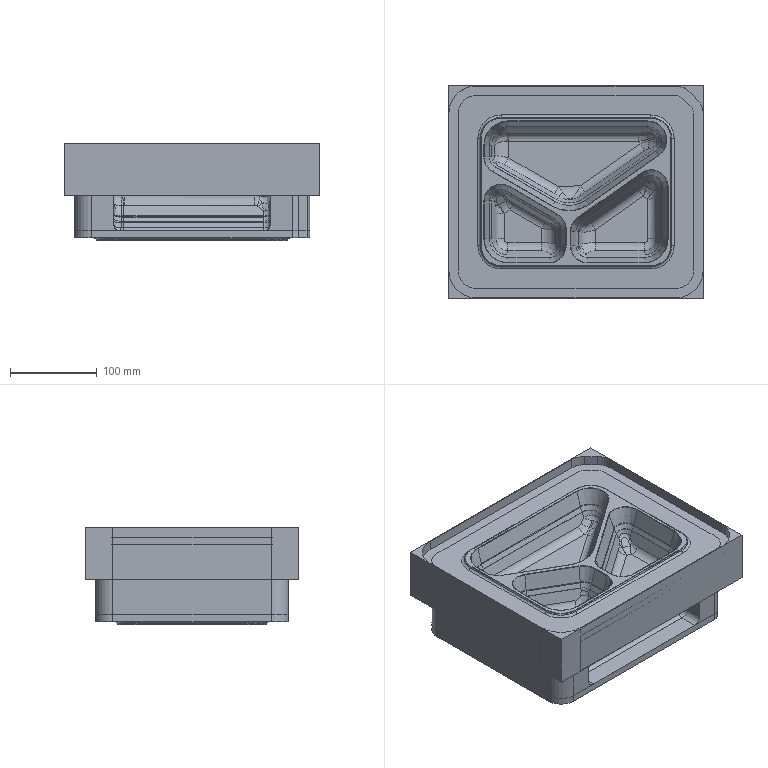Part | 5 solids | 1312 faces | box 295.651 x 246.652 x 112.895 mm | volume 3164635 mm3 | cylinder 344 | plane 293 | spline 252 | cone 215 | torus 207 | sphere 1 | commonest cylinder face diameters 36.004 x49 1.004 x48 20.004 x48 5.996 x33 14.004 x33 30.004 x27